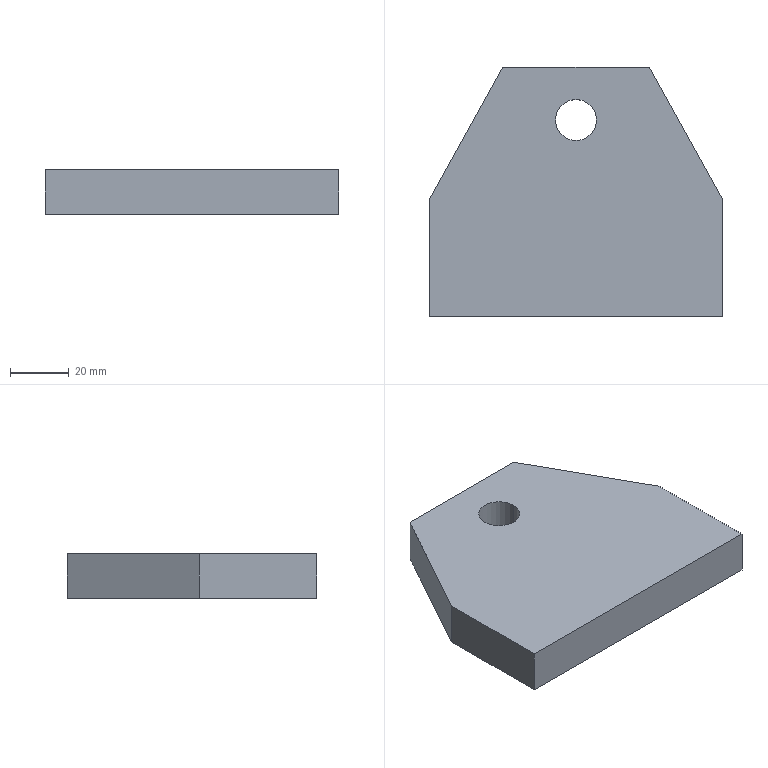Part | SolidWorks | features 3DProfileFeature 1, Extrusion 1, HoleWzd 1 | 1 solid | 10 faces | box 100 x 85 x 15 mm | volume 108316 mm3 | plane 8 | cylinder 2 | commonest cylinder face diameters 14 x2
STEP:
#1=CARTESIAN_POINT('',(-7.,67.,-7.5));
#2=VERTEX_POINT('',#1);
#3=CARTESIAN_POINT('',(7.,67.,-7.5));
#4=VERTEX_POINT('',#3);
#5=CARTESIAN_POINT('',(0.,67.,-7.5));
#6=DIRECTION('',(0.,0.,1.));
#7=DIRECTION('',(1.,0.,0.));
#8=AXIS2_PLACEMENT_3D('',#5,#6,#7);
#9=CIRCLE('',#8,7.);
#10=EDGE_CURVE('',#2,#4,#9,.T.);
#11=ORIENTED_EDGE('',*,*,#10,.F.);
#12=CARTESIAN_POINT('',(-7.,67.,7.5));
#13=VERTEX_POINT('',#12);
#14=CARTESIAN_POINT('',(-7.,67.,7.5));
#15=DIRECTION('',(0.,0.,1.));
#16=VECTOR('',#15,1000.);
#17=LINE('',#14,#16);
#18=EDGE_CURVE('',#2,#13,#17,.T.);
#19=ORIENTED_EDGE('',*,*,#18,.T.);
#20=CARTESIAN_POINT('',(7.,67.,7.5));
#21=VERTEX_POINT('',#20);
#22=CARTESIAN_POINT('',(0.,67.,7.5));
#23=DIRECTION('',(0.,0.,1.));
#24=DIRECTION('',(1.,0.,0.));
#25=AXIS2_PLACEMENT_3D('',#22,#23,#24);
#26=CIRCLE('',#25,7.);
#27=EDGE_CURVE('',#13,#21,#26,.T.);
#28=ORIENTED_EDGE('',*,*,#27,.T.);
#29=CARTESIAN_POINT('',(7.,67.,7.5));
#30=DIRECTION('',(0.,0.,1.));
#31=VECTOR('',#30,1000.);
#32=LINE('',#29,#31);
#33=EDGE_CURVE('',#4,#21,#32,.T.);
#34=ORIENTED_EDGE('',*,*,#33,.F.);
#35=EDGE_LOOP('',(#11,#19,#28,#34));
#36=FACE_OUTER_BOUND('',#35,.T.);
#37=CARTESIAN_POINT('',(0.,67.,7.5));
#38=DIRECTION('',(0.,0.,1.));
#39=DIRECTION('',(1.,0.,0.));
#40=AXIS2_PLACEMENT_3D('',#37,#38,#39);
#41=CYLINDRICAL_SURFACE('',#40,7.);
#42=ADVANCED_FACE('',(#36),#41,.F.);
#43=CARTESIAN_POINT('',(-25.,85.,-7.5));
#44=VERTEX_POINT('',#43);
#45=CARTESIAN_POINT('',(-50.,40.,-7.5));
#46=VERTEX_POINT('',#45);
#47=CARTESIAN_POINT('',(-50.,40.,-7.5));
#48=DIRECTION('',(-0.4856,-0.8742,0.));
#49=VECTOR('',#48,1000.);
#50=LINE('',#47,#49);
#51=EDGE_CURVE('',#44,#46,#50,.T.);
#52=ORIENTED_EDGE('',*,*,#51,.T.);
#53=CARTESIAN_POINT('',(-50.,40.,7.5));
#54=VERTEX_POINT('',#53);
#55=CARTESIAN_POINT('',(-50.,40.,7.5));
#56=DIRECTION('',(0.,0.,-1.));
#57=VECTOR('',#56,1000.);
#58=LINE('',#55,#57);
#59=EDGE_CURVE('',#54,#46,#58,.T.);
#60=ORIENTED_EDGE('',*,*,#59,.F.);
#61=CARTESIAN_POINT('',(-25.,85.,7.5));
#62=VERTEX_POINT('',#61);
#63=CARTESIAN_POINT('',(-50.,40.,7.5));
#64=DIRECTION('',(-0.4856,-0.8742,0.));
#65=VECTOR('',#64,1000.);
#66=LINE('',#63,#65);
#67=EDGE_CURVE('',#62,#54,#66,.T.);
#68=ORIENTED_EDGE('',*,*,#67,.F.);
#69=CARTESIAN_POINT('',(-25.,85.,7.5));
#70=DIRECTION('',(0.,0.,-1.));
#71=VECTOR('',#70,1000.);
#72=LINE('',#69,#71);
#73=EDGE_CURVE('',#62,#44,#72,.T.);
#74=ORIENTED_EDGE('',*,*,#73,.T.);
#75=EDGE_LOOP('',(#52,#60,#68,#74));
#76=FACE_OUTER_BOUND('',#75,.T.);
#77=CARTESIAN_POINT('',(-50.,40.,7.5));
#78=DIRECTION('',(0.8742,-0.4856,0.));
#79=DIRECTION('',(0.4856,0.8742,0.));
#80=AXIS2_PLACEMENT_3D('',#77,#78,#79);
#81=PLANE('',#80);
#82=ADVANCED_FACE('',(#76),#81,.F.);
#83=CARTESIAN_POINT('',(-50.,0.,-7.5));
#84=VERTEX_POINT('',#83);
#85=CARTESIAN_POINT('',(-50.,0.,-7.5));
#86=DIRECTION('',(0.,-1.,0.));
#87=VECTOR('',#86,1000.);
#88=LINE('',#85,#87);
#89=EDGE_CURVE('',#46,#84,#88,.T.);
#90=ORIENTED_EDGE('',*,*,#89,.T.);
#91=CARTESIAN_POINT('',(-50.,0.,7.5));
#92=VERTEX_POINT('',#91);
#93=CARTESIAN_POINT('',(-50.,0.,7.5));
#94=DIRECTION('',(0.,0.,-1.));
#95=VECTOR('',#94,1000.);
#96=LINE('',#93,#95);
#97=EDGE_CURVE('',#92,#84,#96,.T.);
#98=ORIENTED_EDGE('',*,*,#97,.F.);
#99=CARTESIAN_POINT('',(-50.,0.,7.5));
#100=DIRECTION('',(0.,-1.,0.));
#101=VECTOR('',#100,1000.);
#102=LINE('',#99,#101);
#103=EDGE_CURVE('',#54,#92,#102,.T.);
#104=ORIENTED_EDGE('',*,*,#103,.F.);
#105=ORIENTED_EDGE('',*,*,#59,.T.);
#106=EDGE_LOOP('',(#90,#98,#104,#105));
#107=FACE_OUTER_BOUND('',#106,.T.);
#108=CARTESIAN_POINT('',(-50.,0.,7.5));
#109=DIRECTION('',(1.,0.,0.));
#110=DIRECTION('',(0.,0.,-1.));
#111=AXIS2_PLACEMENT_3D('',#108,#109,#110);
#112=PLANE('',#111);
#113=ADVANCED_FACE('',(#107),#112,.F.);
#114=CARTESIAN_POINT('',(50.,0.,-7.5));
#115=VERTEX_POINT('',#114);
#116=CARTESIAN_POINT('',(-50.,0.,-7.5));
#117=DIRECTION('',(1.,0.,0.));
#118=VECTOR('',#117,1000.);
#119=LINE('',#116,#118);
#120=EDGE_CURVE('',#84,#115,#119,.T.);
#121=ORIENTED_EDGE('',*,*,#120,.T.);
#122=CARTESIAN_POINT('',(50.,0.,7.5));
#123=VERTEX_POINT('',#122);
#124=CARTESIAN_POINT('',(50.,0.,7.5));
#125=DIRECTION('',(0.,0.,-1.));
#126=VECTOR('',#125,1000.);
#127=LINE('',#124,#126);
#128=EDGE_CURVE('',#123,#115,#127,.T.);
#129=ORIENTED_EDGE('',*,*,#128,.F.);
#130=CARTESIAN_POINT('',(-50.,0.,7.5));
#131=DIRECTION('',(1.,0.,0.));
#132=VECTOR('',#131,1000.);
#133=LINE('',#130,#132);
#134=EDGE_CURVE('',#92,#123,#133,.T.);
#135=ORIENTED_EDGE('',*,*,#134,.F.);
#136=ORIENTED_EDGE('',*,*,#97,.T.);
#137=EDGE_LOOP('',(#121,#129,#135,#136));
#138=FACE_OUTER_BOUND('',#137,.T.);
#139=CARTESIAN_POINT('',(-50.,0.,7.5));
#140=DIRECTION('',(0.,1.,0.));
#141=DIRECTION('',(0.,0.,1.));
#142=AXIS2_PLACEMENT_3D('',#139,#140,#141);
#143=PLANE('',#142);
#144=ADVANCED_FACE('',(#138),#143,.F.);
#145=CARTESIAN_POINT('',(50.,40.,-7.5));
#146=VERTEX_POINT('',#145);
#147=CARTESIAN_POINT('',(50.,0.,-7.5));
#148=DIRECTION('',(0.,1.,0.));
#149=VECTOR('',#148,1000.);
#150=LINE('',#147,#149);
#151=EDGE_CURVE('',#115,#146,#150,.T.);
#152=ORIENTED_EDGE('',*,*,#151,.T.);
#153=CARTESIAN_POINT('',(50.,40.,7.5));
#154=VERTEX_POINT('',#153);
#155=CARTESIAN_POINT('',(50.,40.,7.5));
#156=DIRECTION('',(0.,0.,-1.));
#157=VECTOR('',#156,1000.);
#158=LINE('',#155,#157);
#159=EDGE_CURVE('',#154,#146,#158,.T.);
#160=ORIENTED_EDGE('',*,*,#159,.F.);
#161=CARTESIAN_POINT('',(50.,0.,7.5));
#162=DIRECTION('',(0.,1.,0.));
#163=VECTOR('',#162,1000.);
#164=LINE('',#161,#163);
#165=EDGE_CURVE('',#123,#154,#164,.T.);
#166=ORIENTED_EDGE('',*,*,#165,.F.);
#167=ORIENTED_EDGE('',*,*,#128,.T.);
#168=EDGE_LOOP('',(#152,#160,#166,#167));
#169=FACE_OUTER_BOUND('',#168,.T.);
#170=CARTESIAN_POINT('',(50.,0.,7.5));
#171=DIRECTION('',(-1.,0.,0.));
#172=DIRECTION('',(0.,0.,1.));
#173=AXIS2_PLACEMENT_3D('',#170,#171,#172);
#174=PLANE('',#173);
#175=ADVANCED_FACE('',(#169),#174,.F.);
#176=CARTESIAN_POINT('',(25.,85.,-7.5));
#177=VERTEX_POINT('',#176);
#178=CARTESIAN_POINT('',(50.,40.,-7.5));
#179=DIRECTION('',(-0.4856,0.8742,0.));
#180=VECTOR('',#179,1000.);
#181=LINE('',#178,#180);
#182=EDGE_CURVE('',#146,#177,#181,.T.);
#183=ORIENTED_EDGE('',*,*,#182,.T.);
#184=CARTESIAN_POINT('',(25.,85.,7.5));
#185=VERTEX_POINT('',#184);
#186=CARTESIAN_POINT('',(25.,85.,7.5));
#187=DIRECTION('',(0.,0.,-1.));
#188=VECTOR('',#187,1000.);
#189=LINE('',#186,#188);
#190=EDGE_CURVE('',#185,#177,#189,.T.);
#191=ORIENTED_EDGE('',*,*,#190,.F.);
#192=CARTESIAN_POINT('',(50.,40.,7.5));
#193=DIRECTION('',(-0.4856,0.8742,0.));
#194=VECTOR('',#193,1000.);
#195=LINE('',#192,#194);
#196=EDGE_CURVE('',#154,#185,#195,.T.);
#197=ORIENTED_EDGE('',*,*,#196,.F.);
#198=ORIENTED_EDGE('',*,*,#159,.T.);
#199=EDGE_LOOP('',(#183,#191,#197,#198));
#200=FACE_OUTER_BOUND('',#199,.T.);
#201=CARTESIAN_POINT('',(50.,40.,7.5));
#202=DIRECTION('',(-0.8742,-0.4856,0.));
#203=DIRECTION('',(0.4856,-0.8742,0.));
#204=AXIS2_PLACEMENT_3D('',#201,#202,#203);
#205=PLANE('',#204);
#206=ADVANCED_FACE('',(#200),#205,.F.);
#207=CARTESIAN_POINT('',(25.,85.,-7.5));
#208=DIRECTION('',(-1.,0.,0.));
#209=VECTOR('',#208,1000.);
#210=LINE('',#207,#209);
#211=EDGE_CURVE('',#177,#44,#210,.T.);
#212=ORIENTED_EDGE('',*,*,#211,.T.);
#213=ORIENTED_EDGE('',*,*,#73,.F.);
#214=CARTESIAN_POINT('',(25.,85.,7.5));
#215=DIRECTION('',(-1.,0.,0.));
#216=VECTOR('',#215,1000.);
#217=LINE('',#214,#216);
#218=EDGE_CURVE('',#185,#62,#217,.T.);
#219=ORIENTED_EDGE('',*,*,#218,.F.);
#220=ORIENTED_EDGE('',*,*,#190,.T.);
#221=EDGE_LOOP('',(#212,#213,#219,#220));
#222=FACE_OUTER_BOUND('',#221,.T.);
#223=CARTESIAN_POINT('',(25.,85.,7.5));
#224=DIRECTION('',(0.,-1.,0.));
#225=DIRECTION('',(0.,0.,-1.));
#226=AXIS2_PLACEMENT_3D('',#223,#224,#225);
#227=PLANE('',#226);
#228=ADVANCED_FACE('',(#222),#227,.F.);
#229=CARTESIAN_POINT('',(0.,67.,7.5));
#230=DIRECTION('',(0.,0.,1.));
#231=DIRECTION('',(1.,0.,0.));
#232=AXIS2_PLACEMENT_3D('',#229,#230,#231);
#233=CIRCLE('',#232,7.);
#234=EDGE_CURVE('',#21,#13,#233,.T.);
#235=ORIENTED_EDGE('',*,*,#234,.F.);
#236=ORIENTED_EDGE('',*,*,#27,.F.);
#237=EDGE_LOOP('',(#235,#236));
#238=FACE_BOUND('',#237,.T.);
#239=ORIENTED_EDGE('',*,*,#67,.T.);
#240=ORIENTED_EDGE('',*,*,#103,.T.);
#241=ORIENTED_EDGE('',*,*,#134,.T.);
#242=ORIENTED_EDGE('',*,*,#165,.T.);
#243=ORIENTED_EDGE('',*,*,#196,.T.);
#244=ORIENTED_EDGE('',*,*,#218,.T.);
#245=EDGE_LOOP('',(#239,#240,#241,#242,#243,#244));
#246=FACE_OUTER_BOUND('',#245,.T.);
#247=CARTESIAN_POINT('',(0.,0.,7.5));
#248=DIRECTION('',(0.,0.,1.));
#249=DIRECTION('',(1.,0.,0.));
#250=AXIS2_PLACEMENT_3D('',#247,#248,#249);
#251=PLANE('',#250);
#252=ADVANCED_FACE('',(#238,#246),#251,.T.);
#253=CARTESIAN_POINT('',(0.,67.,-7.5));
#254=DIRECTION('',(0.,0.,1.));
#255=DIRECTION('',(1.,0.,0.));
#256=AXIS2_PLACEMENT_3D('',#253,#254,#255);
#257=CIRCLE('',#256,7.);
#258=EDGE_CURVE('',#4,#2,#257,.T.);
#259=ORIENTED_EDGE('',*,*,#258,.T.);
#260=ORIENTED_EDGE('',*,*,#10,.T.);
#261=EDGE_LOOP('',(#259,#260));
#262=FACE_BOUND('',#261,.T.);
#263=ORIENTED_EDGE('',*,*,#51,.F.);
#264=ORIENTED_EDGE('',*,*,#211,.F.);
#265=ORIENTED_EDGE('',*,*,#182,.F.);
#266=ORIENTED_EDGE('',*,*,#151,.F.);
#267=ORIENTED_EDGE('',*,*,#120,.F.);
#268=ORIENTED_EDGE('',*,*,#89,.F.);
#269=EDGE_LOOP('',(#263,#264,#265,#266,#267,#268));
#270=FACE_OUTER_BOUND('',#269,.T.);
#271=CARTESIAN_POINT('',(0.,0.,-7.5));
#272=DIRECTION('',(0.,0.,1.));
#273=DIRECTION('',(1.,0.,0.));
#274=AXIS2_PLACEMENT_3D('',#271,#272,#273);
#275=PLANE('',#274);
#276=ADVANCED_FACE('',(#262,#270),#275,.F.);
#277=ORIENTED_EDGE('',*,*,#18,.F.);
#278=ORIENTED_EDGE('',*,*,#258,.F.);
#279=ORIENTED_EDGE('',*,*,#33,.T.);
#280=ORIENTED_EDGE('',*,*,#234,.T.);
#281=EDGE_LOOP('',(#277,#278,#279,#280));
#282=FACE_OUTER_BOUND('',#281,.T.);
#283=CARTESIAN_POINT('',(0.,67.,7.5));
#284=DIRECTION('',(0.,0.,1.));
#285=DIRECTION('',(1.,0.,0.));
#286=AXIS2_PLACEMENT_3D('',#283,#284,#285);
#287=CYLINDRICAL_SURFACE('',#286,7.);
#288=ADVANCED_FACE('',(#282),#287,.F.);
#289=CLOSED_SHELL('',(#42,#82,#113,#144,#175,#206,#228,#252,#276,#288));
#290=MANIFOLD_SOLID_BREP('',#289);
#291=CARTESIAN_POINT('',(0.,0.,0.));
#292=DIRECTION('',(0.,0.,1.));
#293=DIRECTION('',(1.,0.,0.));
#294=AXIS2_PLACEMENT_3D('',#291,#292,#293);
#295=(LENGTH_UNIT()NAMED_UNIT(*)SI_UNIT(.MILLI.,.METRE.));
#296=UNCERTAINTY_MEASURE_WITH_UNIT(LENGTH_MEASURE(0.00001),#295,'','');
#297=(NAMED_UNIT(*)PLANE_ANGLE_UNIT()SI_UNIT($,.RADIAN.));
#298=(NAMED_UNIT(*)SI_UNIT($,.STERADIAN.)SOLID_ANGLE_UNIT());
#299=(GEOMETRIC_REPRESENTATION_CONTEXT(3)GLOBAL_UNCERTAINTY_ASSIGNED_CONTEXT((#296))GLOBAL_UNIT_ASSIGNED_CONTEXT((#295,#297,#298))REPRESENTATION_CONTEXT('',''));
#300=ADVANCED_BREP_SHAPE_REPRESENTATION('',(#290,#294),#299);